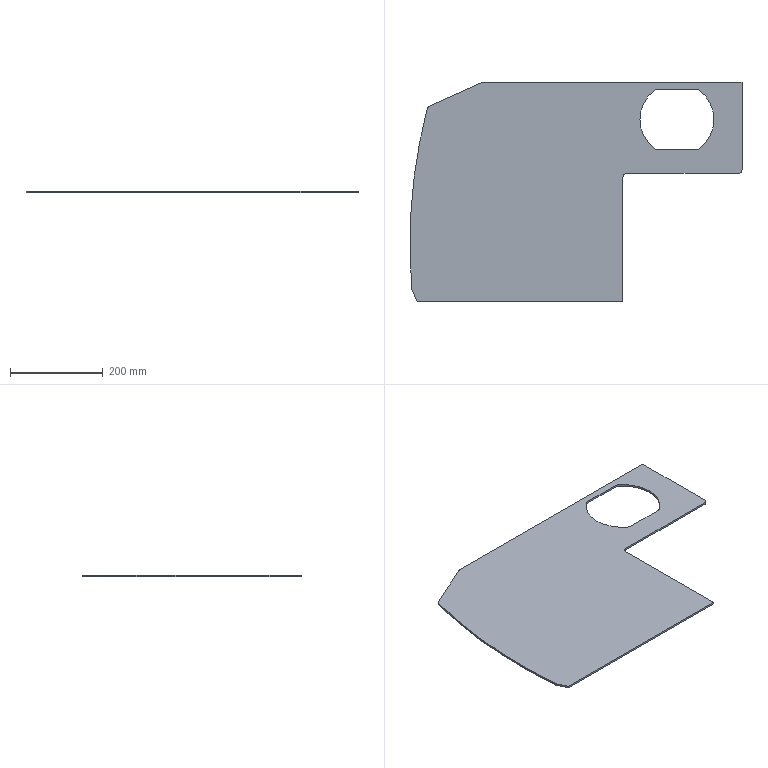Part | SolidWorks | features FlatPattern 1, SMBaseFlange 1, SheetMetal 1 | 1 solid | 24 faces | box 714.283 x 472 x 4 mm | volume 956528 mm3 | cylinder 13 | plane 11 | commonest cylinder face diameters 16 x5 20 x4 159 x3 2302 x1
STEP:
#1=CARTESIAN_POINT('',(-60.5,-80.,-4.));
#2=VERTEX_POINT('',#1);
#3=CARTESIAN_POINT('',(-91.771,-16.8,-4.));
#4=VERTEX_POINT('',#3);
#5=CARTESIAN_POINT('',(-140.,-80.,-4.));
#6=DIRECTION('',(0.,0.,1.));
#7=DIRECTION('',(1.,0.,0.));
#8=AXIS2_PLACEMENT_3D('',#5,#6,#7);
#9=CIRCLE('',#8,79.5);
#10=EDGE_CURVE('',#2,#4,#9,.T.);
#11=ORIENTED_EDGE('',*,*,#10,.F.);
#12=CARTESIAN_POINT('',(-60.5,-80.,0.));
#13=VERTEX_POINT('',#12);
#14=CARTESIAN_POINT('',(-60.5,-80.,-4.));
#15=DIRECTION('',(0.,0.,1.));
#16=VECTOR('',#15,1000.);
#17=LINE('',#14,#16);
#18=EDGE_CURVE('',#2,#13,#17,.T.);
#19=ORIENTED_EDGE('',*,*,#18,.T.);
#20=CARTESIAN_POINT('',(-91.771,-16.8,0.));
#21=VERTEX_POINT('',#20);
#22=CARTESIAN_POINT('',(-140.,-80.,0.));
#23=DIRECTION('',(0.,0.,1.));
#24=DIRECTION('',(1.,0.,0.));
#25=AXIS2_PLACEMENT_3D('',#22,#23,#24);
#26=CIRCLE('',#25,79.5);
#27=EDGE_CURVE('',#13,#21,#26,.T.);
#28=ORIENTED_EDGE('',*,*,#27,.T.);
#29=CARTESIAN_POINT('',(-91.771,-16.8,-4.));
#30=DIRECTION('',(0.,0.,1.));
#31=VECTOR('',#30,1000.);
#32=LINE('',#29,#31);
#33=EDGE_CURVE('',#4,#21,#32,.T.);
#34=ORIENTED_EDGE('',*,*,#33,.F.);
#35=EDGE_LOOP('',(#11,#19,#28,#34));
#36=FACE_OUTER_BOUND('',#35,.T.);
#37=CARTESIAN_POINT('',(-140.,-80.,-4.));
#38=DIRECTION('',(0.,0.,1.));
#39=DIRECTION('',(1.,0.,0.));
#40=AXIS2_PLACEMENT_3D('',#37,#38,#39);
#41=CYLINDRICAL_SURFACE('',#40,79.5);
#42=ADVANCED_FACE('',(#36),#41,.F.);
#43=CARTESIAN_POINT('',(0.,-188.,0.));
#44=VERTEX_POINT('',#43);
#45=CARTESIAN_POINT('',(0.,0.,0.));
#46=VERTEX_POINT('',#45);
#47=CARTESIAN_POINT('',(0.,-188.,0.));
#48=DIRECTION('',(0.,1.,0.));
#49=VECTOR('',#48,1000.);
#50=LINE('',#47,#49);
#51=EDGE_CURVE('',#44,#46,#50,.T.);
#52=ORIENTED_EDGE('',*,*,#51,.F.);
#53=CARTESIAN_POINT('',(0.,-188.,-4.));
#54=VERTEX_POINT('',#53);
#55=CARTESIAN_POINT('',(0.,-188.,-4.));
#56=DIRECTION('',(0.,0.,1.));
#57=VECTOR('',#56,1000.);
#58=LINE('',#55,#57);
#59=EDGE_CURVE('',#54,#44,#58,.T.);
#60=ORIENTED_EDGE('',*,*,#59,.F.);
#61=CARTESIAN_POINT('',(0.,0.,-4.));
#62=VERTEX_POINT('',#61);
#63=CARTESIAN_POINT('',(0.,-188.,-4.));
#64=DIRECTION('',(0.,1.,0.));
#65=VECTOR('',#64,1000.);
#66=LINE('',#63,#65);
#67=EDGE_CURVE('',#54,#62,#66,.T.);
#68=ORIENTED_EDGE('',*,*,#67,.T.);
#69=CARTESIAN_POINT('',(0.,0.,-4.));
#70=DIRECTION('',(0.,0.,1.));
#71=VECTOR('',#70,1000.);
#72=LINE('',#69,#71);
#73=EDGE_CURVE('',#62,#46,#72,.T.);
#74=ORIENTED_EDGE('',*,*,#73,.T.);
#75=EDGE_LOOP('',(#52,#60,#68,#74));
#76=FACE_OUTER_BOUND('',#75,.T.);
#77=CARTESIAN_POINT('',(0.,-188.,-4.));
#78=DIRECTION('',(1.,0.,0.));
#79=DIRECTION('',(0.,0.,-1.));
#80=AXIS2_PLACEMENT_3D('',#77,#78,#79);
#81=PLANE('',#80);
#82=ADVANCED_FACE('',(#76),#81,.T.);
#83=CARTESIAN_POINT('',(-8.,-196.,0.));
#84=VERTEX_POINT('',#83);
#85=CARTESIAN_POINT('',(-8.,-188.,0.));
#86=DIRECTION('',(0.,0.,1.));
#87=DIRECTION('',(1.,0.,0.));
#88=AXIS2_PLACEMENT_3D('',#85,#86,#87);
#89=CIRCLE('',#88,8.);
#90=EDGE_CURVE('',#84,#44,#89,.T.);
#91=ORIENTED_EDGE('',*,*,#90,.F.);
#92=CARTESIAN_POINT('',(-8.,-196.,-4.));
#93=VERTEX_POINT('',#92);
#94=CARTESIAN_POINT('',(-8.,-196.,-4.));
#95=DIRECTION('',(0.,0.,1.));
#96=VECTOR('',#95,1000.);
#97=LINE('',#94,#96);
#98=EDGE_CURVE('',#93,#84,#97,.T.);
#99=ORIENTED_EDGE('',*,*,#98,.F.);
#100=CARTESIAN_POINT('',(-8.,-188.,-4.));
#101=DIRECTION('',(0.,0.,1.));
#102=DIRECTION('',(1.,0.,0.));
#103=AXIS2_PLACEMENT_3D('',#100,#101,#102);
#104=CIRCLE('',#103,8.);
#105=EDGE_CURVE('',#93,#54,#104,.T.);
#106=ORIENTED_EDGE('',*,*,#105,.T.);
#107=ORIENTED_EDGE('',*,*,#59,.T.);
#108=EDGE_LOOP('',(#91,#99,#106,#107));
#109=FACE_OUTER_BOUND('',#108,.T.);
#110=CARTESIAN_POINT('',(-8.,-188.,-4.));
#111=DIRECTION('',(0.,0.,1.));
#112=DIRECTION('',(1.,0.,0.));
#113=AXIS2_PLACEMENT_3D('',#110,#111,#112);
#114=CYLINDRICAL_SURFACE('',#113,8.);
#115=ADVANCED_FACE('',(#109),#114,.T.);
#116=CARTESIAN_POINT('',(-248.,-196.,0.));
#117=VERTEX_POINT('',#116);
#118=CARTESIAN_POINT('',(-248.,-196.,0.));
#119=DIRECTION('',(1.,0.,0.));
#120=VECTOR('',#119,1000.);
#121=LINE('',#118,#120);
#122=EDGE_CURVE('',#117,#84,#121,.T.);
#123=ORIENTED_EDGE('',*,*,#122,.F.);
#124=CARTESIAN_POINT('',(-248.,-196.,-4.));
#125=VERTEX_POINT('',#124);
#126=CARTESIAN_POINT('',(-248.,-196.,-4.));
#127=DIRECTION('',(0.,0.,1.));
#128=VECTOR('',#127,1000.);
#129=LINE('',#126,#128);
#130=EDGE_CURVE('',#125,#117,#129,.T.);
#131=ORIENTED_EDGE('',*,*,#130,.F.);
#132=CARTESIAN_POINT('',(-248.,-196.,-4.));
#133=DIRECTION('',(1.,0.,0.));
#134=VECTOR('',#133,1000.);
#135=LINE('',#132,#134);
#136=EDGE_CURVE('',#125,#93,#135,.T.);
#137=ORIENTED_EDGE('',*,*,#136,.T.);
#138=ORIENTED_EDGE('',*,*,#98,.T.);
#139=EDGE_LOOP('',(#123,#131,#137,#138));
#140=FACE_OUTER_BOUND('',#139,.T.);
#141=CARTESIAN_POINT('',(-248.,-196.,-4.));
#142=DIRECTION('',(0.,-1.,0.));
#143=DIRECTION('',(0.,0.,-1.));
#144=AXIS2_PLACEMENT_3D('',#141,#142,#143);
#145=PLANE('',#144);
#146=ADVANCED_FACE('',(#140),#145,.T.);
#147=CARTESIAN_POINT('',(-256.,-204.,0.));
#148=VERTEX_POINT('',#147);
#149=CARTESIAN_POINT('',(-248.,-204.,0.));
#150=DIRECTION('',(0.,0.,-1.));
#151=DIRECTION('',(-1.,0.,0.));
#152=AXIS2_PLACEMENT_3D('',#149,#150,#151);
#153=CIRCLE('',#152,8.);
#154=EDGE_CURVE('',#148,#117,#153,.T.);
#155=ORIENTED_EDGE('',*,*,#154,.F.);
#156=CARTESIAN_POINT('',(-256.,-204.,-4.));
#157=VERTEX_POINT('',#156);
#158=CARTESIAN_POINT('',(-256.,-204.,-4.));
#159=DIRECTION('',(0.,0.,1.));
#160=VECTOR('',#159,1000.);
#161=LINE('',#158,#160);
#162=EDGE_CURVE('',#157,#148,#161,.T.);
#163=ORIENTED_EDGE('',*,*,#162,.F.);
#164=CARTESIAN_POINT('',(-248.,-204.,-4.));
#165=DIRECTION('',(0.,0.,-1.));
#166=DIRECTION('',(-1.,0.,0.));
#167=AXIS2_PLACEMENT_3D('',#164,#165,#166);
#168=CIRCLE('',#167,8.);
#169=EDGE_CURVE('',#157,#125,#168,.T.);
#170=ORIENTED_EDGE('',*,*,#169,.T.);
#171=ORIENTED_EDGE('',*,*,#130,.T.);
#172=EDGE_LOOP('',(#155,#163,#170,#171));
#173=FACE_OUTER_BOUND('',#172,.T.);
#174=CARTESIAN_POINT('',(-248.,-204.,-4.));
#175=DIRECTION('',(0.,0.,1.));
#176=DIRECTION('',(1.,0.,0.));
#177=AXIS2_PLACEMENT_3D('',#174,#175,#176);
#178=CYLINDRICAL_SURFACE('',#177,8.);
#179=ADVANCED_FACE('',(#173),#178,.F.);
#180=CARTESIAN_POINT('',(-256.,-472.,0.));
#181=VERTEX_POINT('',#180);
#182=CARTESIAN_POINT('',(-256.,-472.,0.));
#183=DIRECTION('',(0.,1.,0.));
#184=VECTOR('',#183,1000.);
#185=LINE('',#182,#184);
#186=EDGE_CURVE('',#181,#148,#185,.T.);
#187=ORIENTED_EDGE('',*,*,#186,.F.);
#188=CARTESIAN_POINT('',(-256.,-472.,-4.));
#189=VERTEX_POINT('',#188);
#190=CARTESIAN_POINT('',(-256.,-472.,-4.));
#191=DIRECTION('',(0.,0.,1.));
#192=VECTOR('',#191,1000.);
#193=LINE('',#190,#192);
#194=EDGE_CURVE('',#189,#181,#193,.T.);
#195=ORIENTED_EDGE('',*,*,#194,.F.);
#196=CARTESIAN_POINT('',(-256.,-472.,-4.));
#197=DIRECTION('',(0.,1.,0.));
#198=VECTOR('',#197,1000.);
#199=LINE('',#196,#198);
#200=EDGE_CURVE('',#189,#157,#199,.T.);
#201=ORIENTED_EDGE('',*,*,#200,.T.);
#202=ORIENTED_EDGE('',*,*,#162,.T.);
#203=EDGE_LOOP('',(#187,#195,#201,#202));
#204=FACE_OUTER_BOUND('',#203,.T.);
#205=CARTESIAN_POINT('',(-256.,-472.,-4.));
#206=DIRECTION('',(1.,0.,0.));
#207=DIRECTION('',(0.,0.,-1.));
#208=AXIS2_PLACEMENT_3D('',#205,#206,#207);
#209=PLANE('',#208);
#210=ADVANCED_FACE('',(#204),#209,.T.);
#211=CARTESIAN_POINT('',(-698.5,-472.,0.));
#212=VERTEX_POINT('',#211);
#213=CARTESIAN_POINT('',(-698.5,-472.,0.));
#214=DIRECTION('',(1.,0.,0.));
#215=VECTOR('',#214,1000.);
#216=LINE('',#213,#215);
#217=EDGE_CURVE('',#212,#181,#216,.T.);
#218=ORIENTED_EDGE('',*,*,#217,.F.);
#219=CARTESIAN_POINT('',(-698.5,-472.,-4.));
#220=VERTEX_POINT('',#219);
#221=CARTESIAN_POINT('',(-698.5,-472.,-4.));
#222=DIRECTION('',(0.,0.,1.));
#223=VECTOR('',#222,1000.);
#224=LINE('',#221,#223);
#225=EDGE_CURVE('',#220,#212,#224,.T.);
#226=ORIENTED_EDGE('',*,*,#225,.F.);
#227=CARTESIAN_POINT('',(-698.5,-472.,-4.));
#228=DIRECTION('',(1.,0.,0.));
#229=VECTOR('',#228,1000.);
#230=LINE('',#227,#229);
#231=EDGE_CURVE('',#220,#189,#230,.T.);
#232=ORIENTED_EDGE('',*,*,#231,.T.);
#233=ORIENTED_EDGE('',*,*,#194,.T.);
#234=EDGE_LOOP('',(#218,#226,#232,#233));
#235=FACE_OUTER_BOUND('',#234,.T.);
#236=CARTESIAN_POINT('',(-698.5,-472.,-4.));
#237=DIRECTION('',(0.,-1.,0.));
#238=DIRECTION('',(1.,0.,0.));
#239=AXIS2_PLACEMENT_3D('',#236,#237,#238);
#240=PLANE('',#239);
#241=ADVANCED_FACE('',(#235),#240,.T.);
#242=CARTESIAN_POINT('',(-709.441,-447.692,0.));
#243=VERTEX_POINT('',#242);
#244=CARTESIAN_POINT('',(-698.5,-472.,0.));
#245=DIRECTION('',(0.4104,-0.9119,0.));
#246=VECTOR('',#245,1000.);
#247=LINE('',#244,#246);
#248=EDGE_CURVE('',#243,#212,#247,.T.);
#249=ORIENTED_EDGE('',*,*,#248,.F.);
#250=CARTESIAN_POINT('',(-709.441,-447.692,-4.));
#251=VERTEX_POINT('',#250);
#252=CARTESIAN_POINT('',(-709.441,-447.692,-4.));
#253=DIRECTION('',(0.,0.,1.));
#254=VECTOR('',#253,1000.);
#255=LINE('',#252,#254);
#256=EDGE_CURVE('',#251,#243,#255,.T.);
#257=ORIENTED_EDGE('',*,*,#256,.F.);
#258=CARTESIAN_POINT('',(-698.5,-472.,-4.));
#259=DIRECTION('',(0.4104,-0.9119,0.));
#260=VECTOR('',#259,1000.);
#261=LINE('',#258,#260);
#262=EDGE_CURVE('',#251,#220,#261,.T.);
#263=ORIENTED_EDGE('',*,*,#262,.T.);
#264=ORIENTED_EDGE('',*,*,#225,.T.);
#265=EDGE_LOOP('',(#249,#257,#263,#264));
#266=FACE_OUTER_BOUND('',#265,.T.);
#267=CARTESIAN_POINT('',(-698.5,-472.,-4.));
#268=DIRECTION('',(-0.9119,-0.4104,0.));
#269=DIRECTION('',(0.4104,-0.9119,0.));
#270=AXIS2_PLACEMENT_3D('',#267,#268,#269);
#271=PLANE('',#270);
#272=ADVANCED_FACE('',(#266),#271,.T.);
#273=CARTESIAN_POINT('',(-710.117,-445.088,0.));
#274=VERTEX_POINT('',#273);
#275=CARTESIAN_POINT('',(-702.146,-444.408,0.));
#276=DIRECTION('',(0.,0.,1.));
#277=DIRECTION('',(-1.,0.,0.));
#278=AXIS2_PLACEMENT_3D('',#275,#276,#277);
#279=CIRCLE('',#278,8.);
#280=EDGE_CURVE('',#274,#243,#279,.T.);
#281=ORIENTED_EDGE('',*,*,#280,.F.);
#282=CARTESIAN_POINT('',(-710.117,-445.088,-4.));
#283=VERTEX_POINT('',#282);
#284=CARTESIAN_POINT('',(-710.117,-445.088,-4.));
#285=DIRECTION('',(0.,0.,1.));
#286=VECTOR('',#285,1000.);
#287=LINE('',#284,#286);
#288=EDGE_CURVE('',#283,#274,#287,.T.);
#289=ORIENTED_EDGE('',*,*,#288,.F.);
#290=CARTESIAN_POINT('',(-702.146,-444.408,-4.));
#291=DIRECTION('',(0.,0.,1.));
#292=DIRECTION('',(-1.,0.,0.));
#293=AXIS2_PLACEMENT_3D('',#290,#291,#292);
#294=CIRCLE('',#293,8.);
#295=EDGE_CURVE('',#283,#251,#294,.T.);
#296=ORIENTED_EDGE('',*,*,#295,.T.);
#297=ORIENTED_EDGE('',*,*,#256,.T.);
#298=EDGE_LOOP('',(#281,#289,#296,#297));
#299=FACE_OUTER_BOUND('',#298,.T.);
#300=CARTESIAN_POINT('',(-702.146,-444.408,-4.));
#301=DIRECTION('',(0.,0.,1.));
#302=DIRECTION('',(1.,0.,0.));
#303=AXIS2_PLACEMENT_3D('',#300,#301,#302);
#304=CYLINDRICAL_SURFACE('',#303,8.);
#305=ADVANCED_FACE('',(#299),#304,.T.);
#306=CARTESIAN_POINT('',(-676.974,-56.578,0.));
#307=VERTEX_POINT('',#306);
#308=CARTESIAN_POINT('',(436.717,-347.252,0.));
#309=DIRECTION('',(0.,0.,1.));
#310=DIRECTION('',(-1.,0.,0.));
#311=AXIS2_PLACEMENT_3D('',#308,#309,#310);
#312=CIRCLE('',#311,1151.);
#313=EDGE_CURVE('',#307,#274,#312,.T.);
#314=ORIENTED_EDGE('',*,*,#313,.F.);
#315=CARTESIAN_POINT('',(-676.974,-56.578,-4.));
#316=VERTEX_POINT('',#315);
#317=CARTESIAN_POINT('',(-676.974,-56.578,-4.));
#318=DIRECTION('',(0.,0.,1.));
#319=VECTOR('',#318,1000.);
#320=LINE('',#317,#319);
#321=EDGE_CURVE('',#316,#307,#320,.T.);
#322=ORIENTED_EDGE('',*,*,#321,.F.);
#323=CARTESIAN_POINT('',(436.717,-347.252,-4.));
#324=DIRECTION('',(0.,0.,1.));
#325=DIRECTION('',(-1.,0.,0.));
#326=AXIS2_PLACEMENT_3D('',#323,#324,#325);
#327=CIRCLE('',#326,1151.);
#328=EDGE_CURVE('',#316,#283,#327,.T.);
#329=ORIENTED_EDGE('',*,*,#328,.T.);
#330=ORIENTED_EDGE('',*,*,#288,.T.);
#331=EDGE_LOOP('',(#314,#322,#329,#330));
#332=FACE_OUTER_BOUND('',#331,.T.);
#333=CARTESIAN_POINT('',(436.717,-347.252,-4.));
#334=DIRECTION('',(0.,0.,1.));
#335=DIRECTION('',(1.,0.,0.));
#336=AXIS2_PLACEMENT_3D('',#333,#334,#335);
#337=CYLINDRICAL_SURFACE('',#336,1151.);
#338=ADVANCED_FACE('',(#332),#337,.T.);
#339=CARTESIAN_POINT('',(-672.516,-51.302,0.));
#340=VERTEX_POINT('',#339);
#341=CARTESIAN_POINT('',(-669.234,-58.598,0.));
#342=DIRECTION('',(0.,0.,1.));
#343=DIRECTION('',(1.,0.,0.));
#344=AXIS2_PLACEMENT_3D('',#341,#342,#343);
#345=CIRCLE('',#344,8.);
#346=EDGE_CURVE('',#340,#307,#345,.T.);
#347=ORIENTED_EDGE('',*,*,#346,.F.);
#348=CARTESIAN_POINT('',(-672.516,-51.302,-4.));
#349=VERTEX_POINT('',#348);
#350=CARTESIAN_POINT('',(-672.516,-51.302,-4.));
#351=DIRECTION('',(0.,0.,1.));
#352=VECTOR('',#351,1000.);
#353=LINE('',#350,#352);
#354=EDGE_CURVE('',#349,#340,#353,.T.);
#355=ORIENTED_EDGE('',*,*,#354,.F.);
#356=CARTESIAN_POINT('',(-669.234,-58.598,-4.));
#357=DIRECTION('',(0.,0.,1.));
#358=DIRECTION('',(1.,0.,0.));
#359=AXIS2_PLACEMENT_3D('',#356,#357,#358);
#360=CIRCLE('',#359,8.);
#361=EDGE_CURVE('',#349,#316,#360,.T.);
#362=ORIENTED_EDGE('',*,*,#361,.T.);
#363=ORIENTED_EDGE('',*,*,#321,.T.);
#364=EDGE_LOOP('',(#347,#355,#362,#363));
#365=FACE_OUTER_BOUND('',#364,.T.);
#366=CARTESIAN_POINT('',(-669.234,-58.598,-4.));
#367=DIRECTION('',(0.,0.,1.));
#368=DIRECTION('',(1.,0.,0.));
#369=AXIS2_PLACEMENT_3D('',#366,#367,#368);
#370=CYLINDRICAL_SURFACE('',#369,8.);
#371=ADVANCED_FACE('',(#365),#370,.T.);
#372=CARTESIAN_POINT('',(-560.066,-0.7045,0.));
#373=VERTEX_POINT('',#372);
#374=CARTESIAN_POINT('',(-560.066,-0.7045,0.));
#375=DIRECTION('',(-0.9119,-0.4103,0.));
#376=VECTOR('',#375,1000.);
#377=LINE('',#374,#376);
#378=EDGE_CURVE('',#373,#340,#377,.T.);
#379=ORIENTED_EDGE('',*,*,#378,.F.);
#380=CARTESIAN_POINT('',(-560.066,-0.7045,-4.));
#381=VERTEX_POINT('',#380);
#382=CARTESIAN_POINT('',(-560.066,-0.7045,-4.));
#383=DIRECTION('',(0.,0.,1.));
#384=VECTOR('',#383,1000.);
#385=LINE('',#382,#384);
#386=EDGE_CURVE('',#381,#373,#385,.T.);
#387=ORIENTED_EDGE('',*,*,#386,.F.);
#388=CARTESIAN_POINT('',(-560.066,-0.7045,-4.));
#389=DIRECTION('',(-0.9119,-0.4103,0.));
#390=VECTOR('',#389,1000.);
#391=LINE('',#388,#390);
#392=EDGE_CURVE('',#381,#349,#391,.T.);
#393=ORIENTED_EDGE('',*,*,#392,.T.);
#394=ORIENTED_EDGE('',*,*,#354,.T.);
#395=EDGE_LOOP('',(#379,#387,#393,#394));
#396=FACE_OUTER_BOUND('',#395,.T.);
#397=CARTESIAN_POINT('',(-560.066,-0.7045,-4.));
#398=DIRECTION('',(-0.4103,0.9119,0.));
#399=DIRECTION('',(-0.9119,-0.4103,0.));
#400=AXIS2_PLACEMENT_3D('',#397,#398,#399);
#401=PLANE('',#400);
#402=ADVANCED_FACE('',(#396),#401,.T.);
#403=CARTESIAN_POINT('',(-556.783,0.,0.));
#404=VERTEX_POINT('',#403);
#405=CARTESIAN_POINT('',(-556.783,-8.,0.));
#406=DIRECTION('',(0.,0.,1.));
#407=DIRECTION('',(1.,0.,0.));
#408=AXIS2_PLACEMENT_3D('',#405,#406,#407);
#409=CIRCLE('',#408,8.);
#410=EDGE_CURVE('',#404,#373,#409,.T.);
#411=ORIENTED_EDGE('',*,*,#410,.F.);
#412=CARTESIAN_POINT('',(-556.783,0.,-4.));
#413=VERTEX_POINT('',#412);
#414=CARTESIAN_POINT('',(-556.783,0.,-4.));
#415=DIRECTION('',(0.,0.,1.));
#416=VECTOR('',#415,1000.);
#417=LINE('',#414,#416);
#418=EDGE_CURVE('',#413,#404,#417,.T.);
#419=ORIENTED_EDGE('',*,*,#418,.F.);
#420=CARTESIAN_POINT('',(-556.783,-8.,-4.));
#421=DIRECTION('',(0.,0.,1.));
#422=DIRECTION('',(1.,0.,0.));
#423=AXIS2_PLACEMENT_3D('',#420,#421,#422);
#424=CIRCLE('',#423,8.);
#425=EDGE_CURVE('',#413,#381,#424,.T.);
#426=ORIENTED_EDGE('',*,*,#425,.T.);
#427=ORIENTED_EDGE('',*,*,#386,.T.);
#428=EDGE_LOOP('',(#411,#419,#426,#427));
#429=FACE_OUTER_BOUND('',#428,.T.);
#430=CARTESIAN_POINT('',(-556.783,-8.,-4.));
#431=DIRECTION('',(0.,0.,1.));
#432=DIRECTION('',(1.,0.,0.));
#433=AXIS2_PLACEMENT_3D('',#430,#431,#432);
#434=CYLINDRICAL_SURFACE('',#433,8.);
#435=ADVANCED_FACE('',(#429),#434,.T.);
#436=CARTESIAN_POINT('',(0.,0.,0.));
#437=DIRECTION('',(-1.,0.,0.));
#438=VECTOR('',#437,1000.);
#439=LINE('',#436,#438);
#440=EDGE_CURVE('',#46,#404,#439,.T.);
#441=ORIENTED_EDGE('',*,*,#440,.F.);
#442=ORIENTED_EDGE('',*,*,#73,.F.);
#443=CARTESIAN_POINT('',(0.,0.,-4.));
#444=DIRECTION('',(-1.,0.,0.));
#445=VECTOR('',#444,1000.);
#446=LINE('',#443,#445);
#447=EDGE_CURVE('',#62,#413,#446,.T.);
#448=ORIENTED_EDGE('',*,*,#447,.T.);
#449=ORIENTED_EDGE('',*,*,#418,.T.);
#450=EDGE_LOOP('',(#441,#442,#448,#449));
#451=FACE_OUTER_BOUND('',#450,.T.);
#452=CARTESIAN_POINT('',(0.,0.,-4.));
#453=DIRECTION('',(0.,1.,0.));
#454=DIRECTION('',(-1.,0.,0.));
#455=AXIS2_PLACEMENT_3D('',#452,#453,#454);
#456=PLANE('',#455);
#457=ADVANCED_FACE('',(#451),#456,.T.);
#458=CARTESIAN_POINT('',(-188.229,-16.8,-4.));
#459=VERTEX_POINT('',#458);
#460=CARTESIAN_POINT('',(-188.229,-143.2,-4.));
#461=VERTEX_POINT('',#460);
#462=CARTESIAN_POINT('',(-140.,-80.,-4.));
#463=DIRECTION('',(0.,0.,1.));
#464=DIRECTION('',(1.,0.,0.));
#465=AXIS2_PLACEMENT_3D('',#462,#463,#464);
#466=CIRCLE('',#465,79.5);
#467=EDGE_CURVE('',#459,#461,#466,.T.);
#468=ORIENTED_EDGE('',*,*,#467,.T.);
#469=CARTESIAN_POINT('',(-182.163,-145.25,-4.));
#470=VERTEX_POINT('',#469);
#471=CARTESIAN_POINT('',(-182.163,-135.25,-4.));
#472=DIRECTION('',(0.,0.,1.));
#473=DIRECTION('',(-1.,0.,0.));
#474=AXIS2_PLACEMENT_3D('',#471,#472,#473);
#475=CIRCLE('',#474,10.);
#476=EDGE_CURVE('',#461,#470,#475,.T.);
#477=ORIENTED_EDGE('',*,*,#476,.T.);
#478=CARTESIAN_POINT('',(-97.837,-145.25,-4.));
#479=VERTEX_POINT('',#478);
#480=CARTESIAN_POINT('',(-182.163,-145.25,-4.));
#481=DIRECTION('',(1.,0.,0.));
#482=VECTOR('',#481,1000.);
#483=LINE('',#480,#482);
#484=EDGE_CURVE('',#470,#479,#483,.T.);
#485=ORIENTED_EDGE('',*,*,#484,.T.);
#486=CARTESIAN_POINT('',(-91.771,-143.2,-4.));
#487=VERTEX_POINT('',#486);
#488=CARTESIAN_POINT('',(-97.837,-135.25,-4.));
#489=DIRECTION('',(0.,0.,1.));
#490=DIRECTION('',(1.,0.,0.));
#491=AXIS2_PLACEMENT_3D('',#488,#489,#490);
#492=CIRCLE('',#491,10.);
#493=EDGE_CURVE('',#479,#487,#492,.T.);
#494=ORIENTED_EDGE('',*,*,#493,.T.);
#495=CARTESIAN_POINT('',(-140.,-80.,-4.));
#496=DIRECTION('',(0.,0.,1.));
#497=DIRECTION('',(1.,0.,0.));
#498=AXIS2_PLACEMENT_3D('',#495,#496,#497);
#499=CIRCLE('',#498,79.5);
#500=EDGE_CURVE('',#487,#2,#499,.T.);
#501=ORIENTED_EDGE('',*,*,#500,.T.);
#502=ORIENTED_EDGE('',*,*,#10,.T.);
#503=CARTESIAN_POINT('',(-97.837,-14.75,-4.));
#504=VERTEX_POINT('',#503);
#505=CARTESIAN_POINT('',(-97.837,-24.75,-4.));
#506=DIRECTION('',(0.,0.,1.));
#507=DIRECTION('',(-1.,0.,0.));
#508=AXIS2_PLACEMENT_3D('',#505,#506,#507);
#509=CIRCLE('',#508,10.);
#510=EDGE_CURVE('',#4,#504,#509,.T.);
#511=ORIENTED_EDGE('',*,*,#510,.T.);
#512=CARTESIAN_POINT('',(-182.163,-14.75,-4.));
#513=VERTEX_POINT('',#512);
#514=CARTESIAN_POINT('',(-182.163,-14.75,-4.));
#515=DIRECTION('',(-1.,0.,0.));
#516=VECTOR('',#515,1000.);
#517=LINE('',#514,#516);
#518=EDGE_CURVE('',#504,#513,#517,.T.);
#519=ORIENTED_EDGE('',*,*,#518,.T.);
#520=CARTESIAN_POINT('',(-182.163,-24.75,-4.));
#521=DIRECTION('',(0.,0.,1.));
#522=DIRECTION('',(1.,0.,0.));
#523=AXIS2_PLACEMENT_3D('',#520,#521,#522);
#524=CIRCLE('',#523,10.);
#525=EDGE_CURVE('',#513,#459,#524,.T.);
#526=ORIENTED_EDGE('',*,*,#525,.T.);
#527=EDGE_LOOP('',(#468,#477,#485,#494,#501,#502,#511,#519,#526));
#528=FACE_BOUND('',#527,.T.);
#529=ORIENTED_EDGE('',*,*,#67,.F.);
#530=ORIENTED_EDGE('',*,*,#105,.F.);
#531=ORIENTED_EDGE('',*,*,#136,.F.);
#532=ORIENTED_EDGE('',*,*,#169,.F.);
#533=ORIENTED_EDGE('',*,*,#200,.F.);
#534=ORIENTED_EDGE('',*,*,#231,.F.);
#535=ORIENTED_EDGE('',*,*,#262,.F.);
#536=ORIENTED_EDGE('',*,*,#295,.F.);
#537=ORIENTED_EDGE('',*,*,#328,.F.);
#538=ORIENTED_EDGE('',*,*,#361,.F.);
#539=ORIENTED_EDGE('',*,*,#392,.F.);
#540=ORIENTED_EDGE('',*,*,#425,.F.);
#541=ORIENTED_EDGE('',*,*,#447,.F.);
#542=EDGE_LOOP('',(#529,#530,#531,#532,#533,#534,#535,#536,#537,#538,#539,#540,#541));
#543=FACE_OUTER_BOUND('',#542,.T.);
#544=CARTESIAN_POINT('',(-556.783,-8.,-4.));
#545=DIRECTION('',(0.,0.,1.));
#546=DIRECTION('',(1.,0.,0.));
#547=AXIS2_PLACEMENT_3D('',#544,#545,#546);
#548=PLANE('',#547);
#549=ADVANCED_FACE('',(#528,#543),#548,.F.);
#550=CARTESIAN_POINT('',(-188.229,-143.2,0.));
#551=VERTEX_POINT('',#550);
#552=CARTESIAN_POINT('',(-182.163,-145.25,0.));
#553=VERTEX_POINT('',#552);
#554=CARTESIAN_POINT('',(-182.163,-135.25,0.));
#555=DIRECTION('',(0.,0.,1.));
#556=DIRECTION('',(-1.,0.,0.));
#557=AXIS2_PLACEMENT_3D('',#554,#555,#556);
#558=CIRCLE('',#557,10.);
#559=EDGE_CURVE('',#551,#553,#558,.T.);
#560=ORIENTED_EDGE('',*,*,#559,.F.);
#561=CARTESIAN_POINT('',(-188.229,-16.8,0.));
#562=VERTEX_POINT('',#561);
#563=CARTESIAN_POINT('',(-140.,-80.,0.));
#564=DIRECTION('',(0.,0.,1.));
#565=DIRECTION('',(1.,0.,0.));
#566=AXIS2_PLACEMENT_3D('',#563,#564,#565);
#567=CIRCLE('',#566,79.5);
#568=EDGE_CURVE('',#562,#551,#567,.T.);
#569=ORIENTED_EDGE('',*,*,#568,.F.);
#570=CARTESIAN_POINT('',(-182.163,-14.75,0.));
#571=VERTEX_POINT('',#570);
#572=CARTESIAN_POINT('',(-182.163,-24.75,0.));
#573=DIRECTION('',(0.,0.,1.));
#574=DIRECTION('',(1.,0.,0.));
#575=AXIS2_PLACEMENT_3D('',#572,#573,#574);
#576=CIRCLE('',#575,10.);
#577=EDGE_CURVE('',#571,#562,#576,.T.);
#578=ORIENTED_EDGE('',*,*,#577,.F.);
#579=CARTESIAN_POINT('',(-97.837,-14.75,0.));
#580=VERTEX_POINT('',#579);
#581=CARTESIAN_POINT('',(-182.163,-14.75,0.));
#582=DIRECTION('',(-1.,0.,0.));
#583=VECTOR('',#582,1000.);
#584=LINE('',#581,#583);
#585=EDGE_CURVE('',#580,#571,#584,.T.);
#586=ORIENTED_EDGE('',*,*,#585,.F.);
#587=CARTESIAN_POINT('',(-97.837,-24.75,0.));
#588=DIRECTION('',(0.,0.,1.));
#589=DIRECTION('',(-1.,0.,0.));
#590=AXIS2_PLACEMENT_3D('',#587,#588,#589);
#591=CIRCLE('',#590,10.);
#592=EDGE_CURVE('',#21,#580,#591,.T.);
#593=ORIENTED_EDGE('',*,*,#592,.F.);
#594=ORIENTED_EDGE('',*,*,#27,.F.);
#595=CARTESIAN_POINT('',(-91.771,-143.2,0.));
#596=VERTEX_POINT('',#595);
#597=CARTESIAN_POINT('',(-140.,-80.,0.));
#598=DIRECTION('',(0.,0.,1.));
#599=DIRECTION('',(1.,0.,0.));
#600=AXIS2_PLACEMENT_3D('',#597,#598,#599);
#601=CIRCLE('',#600,79.5);
#602=EDGE_CURVE('',#596,#13,#601,.T.);
#603=ORIENTED_EDGE('',*,*,#602,.F.);
#604=CARTESIAN_POINT('',(-97.837,-145.25,0.));
#605=VERTEX_POINT('',#604);
#606=CARTESIAN_POINT('',(-97.837,-135.25,0.));
#607=DIRECTION('',(0.,0.,1.));
#608=DIRECTION('',(1.,0.,0.));
#609=AXIS2_PLACEMENT_3D('',#606,#607,#608);
#610=CIRCLE('',#609,10.);
#611=EDGE_CURVE('',#605,#596,#610,.T.);
#612=ORIENTED_EDGE('',*,*,#611,.F.);
#613=CARTESIAN_POINT('',(-182.163,-145.25,0.));
#614=DIRECTION('',(1.,0.,0.));
#615=VECTOR('',#614,1000.);
#616=LINE('',#613,#615);
#617=EDGE_CURVE('',#553,#605,#616,.T.);
#618=ORIENTED_EDGE('',*,*,#617,.F.);
#619=EDGE_LOOP('',(#560,#569,#578,#586,#593,#594,#603,#612,#618));
#620=FACE_BOUND('',#619,.T.);
#621=ORIENTED_EDGE('',*,*,#51,.T.);
#622=ORIENTED_EDGE('',*,*,#440,.T.);
#623=ORIENTED_EDGE('',*,*,#410,.T.);
#624=ORIENTED_EDGE('',*,*,#378,.T.);
#625=ORIENTED_EDGE('',*,*,#346,.T.);
#626=ORIENTED_EDGE('',*,*,#313,.T.);
#627=ORIENTED_EDGE('',*,*,#280,.T.);
#628=ORIENTED_EDGE('',*,*,#248,.T.);
#629=ORIENTED_EDGE('',*,*,#217,.T.);
#630=ORIENTED_EDGE('',*,*,#186,.T.);
#631=ORIENTED_EDGE('',*,*,#154,.T.);
#632=ORIENTED_EDGE('',*,*,#122,.T.);
#633=ORIENTED_EDGE('',*,*,#90,.T.);
#634=EDGE_LOOP('',(#621,#622,#623,#624,#625,#626,#627,#628,#629,#630,#631,#632,#633));
#635=FACE_OUTER_BOUND('',#634,.T.);
#636=CARTESIAN_POINT('',(-556.783,-8.,0.));
#637=DIRECTION('',(0.,0.,1.));
#638=DIRECTION('',(1.,0.,0.));
#639=AXIS2_PLACEMENT_3D('',#636,#637,#638);
#640=PLANE('',#639);
#641=ADVANCED_FACE('',(#620,#635),#640,.T.);
#642=ORIENTED_EDGE('',*,*,#559,.T.);
#643=CARTESIAN_POINT('',(-182.163,-145.25,-4.));
#644=DIRECTION('',(0.,0.,1.));
#645=VECTOR('',#644,1000.);
#646=LINE('',#643,#645);
#647=EDGE_CURVE('',#470,#553,#646,.T.);
#648=ORIENTED_EDGE('',*,*,#647,.F.);
#649=ORIENTED_EDGE('',*,*,#476,.F.);
#650=CARTESIAN_POINT('',(-188.229,-143.2,-4.));
#651=DIRECTION('',(0.,0.,1.));
#652=VECTOR('',#651,1000.);
#653=LINE('',#650,#652);
#654=EDGE_CURVE('',#461,#551,#653,.T.);
#655=ORIENTED_EDGE('',*,*,#654,.T.);
#656=EDGE_LOOP('',(#642,#648,#649,#655));
#657=FACE_OUTER_BOUND('',#656,.T.);
#658=CARTESIAN_POINT('',(-182.163,-135.25,-4.));
#659=DIRECTION('',(0.,0.,1.));
#660=DIRECTION('',(1.,0.,0.));
#661=AXIS2_PLACEMENT_3D('',#658,#659,#660);
#662=CYLINDRICAL_SURFACE('',#661,10.);
#663=ADVANCED_FACE('',(#657),#662,.F.);
#664=ORIENTED_EDGE('',*,*,#568,.T.);
#665=ORIENTED_EDGE('',*,*,#654,.F.);
#666=ORIENTED_EDGE('',*,*,#467,.F.);
#667=CARTESIAN_POINT('',(-188.229,-16.8,-4.));
#668=DIRECTION('',(0.,0.,1.));
#669=VECTOR('',#668,1000.);
#670=LINE('',#667,#669);
#671=EDGE_CURVE('',#459,#562,#670,.T.);
#672=ORIENTED_EDGE('',*,*,#671,.T.);
#673=EDGE_LOOP('',(#664,#665,#666,#672));
#674=FACE_OUTER_BOUND('',#673,.T.);
#675=CARTESIAN_POINT('',(-140.,-80.,-4.));
#676=DIRECTION('',(0.,0.,1.));
#677=DIRECTION('',(1.,0.,0.));
#678=AXIS2_PLACEMENT_3D('',#675,#676,#677);
#679=CYLINDRICAL_SURFACE('',#678,79.5);
#680=ADVANCED_FACE('',(#674),#679,.F.);
#681=ORIENTED_EDGE('',*,*,#577,.T.);
#682=ORIENTED_EDGE('',*,*,#671,.F.);
#683=ORIENTED_EDGE('',*,*,#525,.F.);
#684=CARTESIAN_POINT('',(-182.163,-14.75,-4.));
#685=DIRECTION('',(0.,0.,1.));
#686=VECTOR('',#685,1000.);
#687=LINE('',#684,#686);
#688=EDGE_CURVE('',#513,#571,#687,.T.);
#689=ORIENTED_EDGE('',*,*,#688,.T.);
#690=EDGE_LOOP('',(#681,#682,#683,#689));
#691=FACE_OUTER_BOUND('',#690,.T.);
#692=CARTESIAN_POINT('',(-182.163,-24.75,-4.));
#693=DIRECTION('',(0.,0.,1.));
#694=DIRECTION('',(1.,0.,0.));
#695=AXIS2_PLACEMENT_3D('',#692,#693,#694);
#696=CYLINDRICAL_SURFACE('',#695,10.);
#697=ADVANCED_FACE('',(#691),#696,.F.);
#698=ORIENTED_EDGE('',*,*,#585,.T.);
#699=ORIENTED_EDGE('',*,*,#688,.F.);
#700=ORIENTED_EDGE('',*,*,#518,.F.);
#701=CARTESIAN_POINT('',(-97.837,-14.75,-4.));
#702=DIRECTION('',(0.,0.,1.));
#703=VECTOR('',#702,1000.);
#704=LINE('',#701,#703);
#705=EDGE_CURVE('',#504,#580,#704,.T.);
#706=ORIENTED_EDGE('',*,*,#705,.T.);
#707=EDGE_LOOP('',(#698,#699,#700,#706));
#708=FACE_OUTER_BOUND('',#707,.T.);
#709=CARTESIAN_POINT('',(-182.163,-14.75,-4.));
#710=DIRECTION('',(0.,1.,0.));
#711=DIRECTION('',(-1.,0.,0.));
#712=AXIS2_PLACEMENT_3D('',#709,#710,#711);
#713=PLANE('',#712);
#714=ADVANCED_FACE('',(#708),#713,.F.);
#715=ORIENTED_EDGE('',*,*,#592,.T.);
#716=ORIENTED_EDGE('',*,*,#705,.F.);
#717=ORIENTED_EDGE('',*,*,#510,.F.);
#718=ORIENTED_EDGE('',*,*,#33,.T.);
#719=EDGE_LOOP('',(#715,#716,#717,#718));
#720=FACE_OUTER_BOUND('',#719,.T.);
#721=CARTESIAN_POINT('',(-97.837,-24.75,-4.));
#722=DIRECTION('',(0.,0.,1.));
#723=DIRECTION('',(1.,0.,0.));
#724=AXIS2_PLACEMENT_3D('',#721,#722,#723);
#725=CYLINDRICAL_SURFACE('',#724,10.);
#726=ADVANCED_FACE('',(#720),#725,.F.);
#727=ORIENTED_EDGE('',*,*,#18,.F.);
#728=ORIENTED_EDGE('',*,*,#500,.F.);
#729=CARTESIAN_POINT('',(-91.771,-143.2,-4.));
#730=DIRECTION('',(0.,0.,1.));
#731=VECTOR('',#730,1000.);
#732=LINE('',#729,#731);
#733=EDGE_CURVE('',#487,#596,#732,.T.);
#734=ORIENTED_EDGE('',*,*,#733,.T.);
#735=ORIENTED_EDGE('',*,*,#602,.T.);
#736=EDGE_LOOP('',(#727,#728,#734,#735));
#737=FACE_OUTER_BOUND('',#736,.T.);
#738=CARTESIAN_POINT('',(-140.,-80.,-4.));
#739=DIRECTION('',(0.,0.,1.));
#740=DIRECTION('',(1.,0.,0.));
#741=AXIS2_PLACEMENT_3D('',#738,#739,#740);
#742=CYLINDRICAL_SURFACE('',#741,79.5);
#743=ADVANCED_FACE('',(#737),#742,.F.);
#744=ORIENTED_EDGE('',*,*,#611,.T.);
#745=ORIENTED_EDGE('',*,*,#733,.F.);
#746=ORIENTED_EDGE('',*,*,#493,.F.);
#747=CARTESIAN_POINT('',(-97.837,-145.25,-4.));
#748=DIRECTION('',(0.,0.,1.));
#749=VECTOR('',#748,1000.);
#750=LINE('',#747,#749);
#751=EDGE_CURVE('',#479,#605,#750,.T.);
#752=ORIENTED_EDGE('',*,*,#751,.T.);
#753=EDGE_LOOP('',(#744,#745,#746,#752));
#754=FACE_OUTER_BOUND('',#753,.T.);
#755=CARTESIAN_POINT('',(-97.837,-135.25,-4.));
#756=DIRECTION('',(0.,0.,1.));
#757=DIRECTION('',(1.,0.,0.));
#758=AXIS2_PLACEMENT_3D('',#755,#756,#757);
#759=CYLINDRICAL_SURFACE('',#758,10.);
#760=ADVANCED_FACE('',(#754),#759,.F.);
#761=ORIENTED_EDGE('',*,*,#617,.T.);
#762=ORIENTED_EDGE('',*,*,#751,.F.);
#763=ORIENTED_EDGE('',*,*,#484,.F.);
#764=ORIENTED_EDGE('',*,*,#647,.T.);
#765=EDGE_LOOP('',(#761,#762,#763,#764));
#766=FACE_OUTER_BOUND('',#765,.T.);
#767=CARTESIAN_POINT('',(-182.163,-145.25,-4.));
#768=DIRECTION('',(0.,-1.,0.));
#769=DIRECTION('',(1.,0.,0.));
#770=AXIS2_PLACEMENT_3D('',#767,#768,#769);
#771=PLANE('',#770);
#772=ADVANCED_FACE('',(#766),#771,.F.);
#773=CLOSED_SHELL('',(#42,#82,#115,#146,#179,#210,#241,#272,#305,#338,#371,#402,#435,#457,#549,#641,#663,#680,#697,#714,#726,#743,#760,#772));
#774=MANIFOLD_SOLID_BREP('',#773);
#775=CARTESIAN_POINT('',(0.,0.,0.));
#776=DIRECTION('',(0.,0.,1.));
#777=DIRECTION('',(1.,0.,0.));
#778=AXIS2_PLACEMENT_3D('',#775,#776,#777);
#779=(LENGTH_UNIT()NAMED_UNIT(*)SI_UNIT(.MILLI.,.METRE.));
#780=UNCERTAINTY_MEASURE_WITH_UNIT(LENGTH_MEASURE(0.00001),#779,'','');
#781=(NAMED_UNIT(*)PLANE_ANGLE_UNIT()SI_UNIT($,.RADIAN.));
#782=(NAMED_UNIT(*)SI_UNIT($,.STERADIAN.)SOLID_ANGLE_UNIT());
#783=(GEOMETRIC_REPRESENTATION_CONTEXT(3)GLOBAL_UNCERTAINTY_ASSIGNED_CONTEXT((#780))GLOBAL_UNIT_ASSIGNED_CONTEXT((#779,#781,#782))REPRESENTATION_CONTEXT('',''));
#784=ADVANCED_BREP_SHAPE_REPRESENTATION('',(#774,#778),#783);